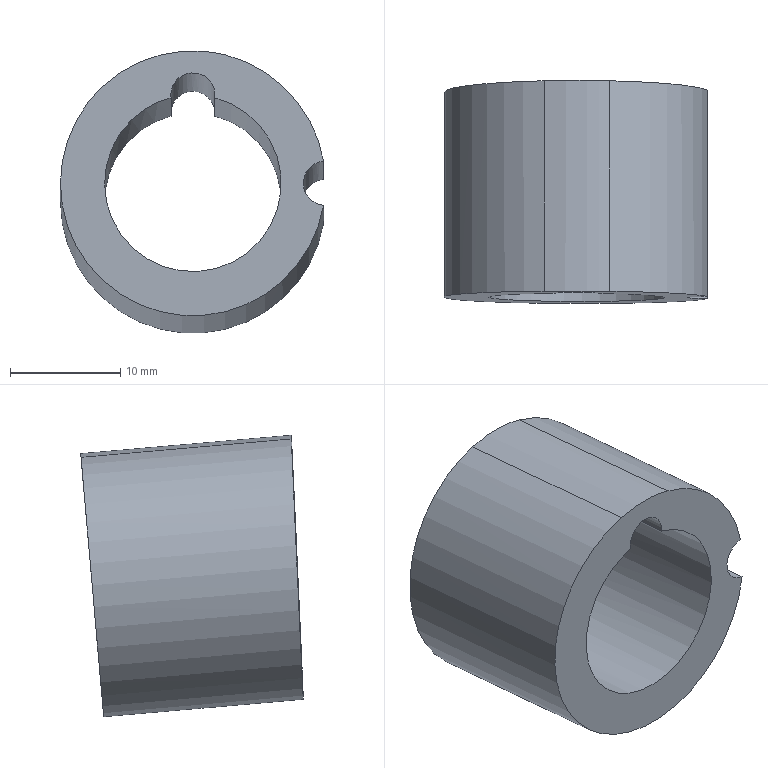Part | NX | features solid 2 | 1 solid | 8 faces | box 23.833 x 20.172 x 25.577 mm | volume 4448 mm3 | cylinder 5 | plane 2 | spline 1 | commonest cylinder face diameters 4 x2 24 x2 16 x1
STEP:
#1=CARTESIAN_POINT('',(82.605,-45.903,-31.729));
#2=VERTEX_POINT('',#1);
#3=CARTESIAN_POINT('',(91.462,-46.359,-41.358));
#4=VERTEX_POINT('',#3);
#5=CARTESIAN_POINT('',(79.629,-46.426,-43.353));
#6=DIRECTION('',(0.001957,0.999,-0.04546));
#7=DIRECTION('',(0.04675,0.04532,0.9979));
#8=AXIS2_PLACEMENT_3D('',#5,#6,#7);
#9=ELLIPSE('',#8,12.011,12.);
#10=EDGE_CURVE('',#2,#4,#9,.T.);
#11=ORIENTED_EDGE('',*,*,#10,.T.);
#12=CARTESIAN_POINT('',(91.462,-27.673,-42.993));
#13=VERTEX_POINT('',#12);
#14=CARTESIAN_POINT('',(91.462,-37.072,-42.17));
#15=DIRECTION('',(0.,0.9962,-0.08716));
#16=VECTOR('',#15,1000.);
#17=LINE('',#14,#16);
#18=EDGE_CURVE('',#4,#13,#17,.T.);
#19=ORIENTED_EDGE('',*,*,#18,.T.);
#20=CARTESIAN_POINT('',(82.605,-26.833,-33.397));
#21=VERTEX_POINT('',#20);
#22=CARTESIAN_POINT('',(79.629,-27.846,-44.978));
#23=DIRECTION('',(0.,0.9962,-0.08716));
#24=DIRECTION('',(0.,0.08716,0.9962));
#25=AXIS2_PLACEMENT_3D('',#22,#23,#24);
#26=CIRCLE('',#25,12.);
#27=EDGE_CURVE('',#21,#13,#26,.T.);
#28=ORIENTED_EDGE('',*,*,#27,.F.);
#29=CARTESIAN_POINT('',(82.605,-26.833,-33.397));
#30=DIRECTION('',(0.,-0.9962,0.08716));
#31=VECTOR('',#30,1000.);
#32=LINE('',#29,#31);
#33=EDGE_CURVE('',#21,#2,#32,.T.);
#34=ORIENTED_EDGE('',*,*,#33,.T.);
#35=EDGE_LOOP('',(#11,#19,#28,#34));
#36=FACE_BOUND('',#35,.T.);
#37=CARTESIAN_POINT('',(79.629,-27.846,-44.978));
#38=DIRECTION('',(0.,-0.9962,0.08716));
#39=DIRECTION('',(0.,-0.08716,-0.9962));
#40=AXIS2_PLACEMENT_3D('',#37,#38,#39);
#41=CYLINDRICAL_SURFACE('',#40,12.);
#42=ADVANCED_FACE('',(#36),#41,.T.);
#43=CARTESIAN_POINT('',(81.613,-46.077,-35.604));
#44=VERTEX_POINT('',#43);
#45=CARTESIAN_POINT('',(77.644,-46.07,-35.604));
#46=VERTEX_POINT('',#45);
#47=CARTESIAN_POINT('',(79.629,-46.426,-43.353));
#48=DIRECTION('',(0.001957,0.999,-0.04546));
#49=DIRECTION('',(0.04675,0.04532,0.9979));
#50=AXIS2_PLACEMENT_3D('',#47,#48,#49);
#51=ELLIPSE('',#50,8.007,8.);
#52=EDGE_CURVE('',#44,#46,#51,.T.);
#53=ORIENTED_EDGE('',*,*,#52,.F.);
#54=CARTESIAN_POINT('',(81.613,-27.171,-37.258));
#55=VERTEX_POINT('',#54);
#56=CARTESIAN_POINT('',(81.613,-27.171,-37.258));
#57=DIRECTION('',(0.,-0.9962,0.08716));
#58=VECTOR('',#57,1000.);
#59=LINE('',#56,#58);
#60=EDGE_CURVE('',#55,#44,#59,.T.);
#61=ORIENTED_EDGE('',*,*,#60,.F.);
#62=CARTESIAN_POINT('',(77.644,-27.171,-37.258));
#63=VERTEX_POINT('',#62);
#64=CARTESIAN_POINT('',(79.629,-27.846,-44.978));
#65=DIRECTION('',(0.,-0.9962,0.08716));
#66=DIRECTION('',(0.,-0.08716,-0.9962));
#67=AXIS2_PLACEMENT_3D('',#64,#65,#66);
#68=CIRCLE('',#67,8.);
#69=EDGE_CURVE('',#55,#63,#68,.F.);
#70=ORIENTED_EDGE('',*,*,#69,.T.);
#71=CARTESIAN_POINT('',(77.644,-27.171,-37.258));
#72=DIRECTION('',(0.,-0.9962,0.08716));
#73=VECTOR('',#72,1000.);
#74=LINE('',#71,#73);
#75=EDGE_CURVE('',#46,#63,#74,.F.);
#76=ORIENTED_EDGE('',*,*,#75,.F.);
#77=EDGE_LOOP('',(#53,#61,#70,#76));
#78=FACE_BOUND('',#77,.T.);
#79=CARTESIAN_POINT('',(79.629,-27.846,-44.978));
#80=DIRECTION('',(0.,-0.9962,0.08716));
#81=DIRECTION('',(0.,-0.08716,-0.9962));
#82=AXIS2_PLACEMENT_3D('',#79,#80,#81);
#83=CYLINDRICAL_SURFACE('',#82,8.);
#84=ADVANCED_FACE('',(#78),#83,.F.);
#85=CARTESIAN_POINT('',(91.462,-28.02,-46.964));
#86=VERTEX_POINT('',#85);
#87=CARTESIAN_POINT('',(91.629,-27.846,-44.978));
#88=DIRECTION('',(0.,-0.9962,0.08716));
#89=DIRECTION('',(0.,-0.08716,-0.9962));
#90=AXIS2_PLACEMENT_3D('',#87,#88,#89);
#91=CIRCLE('',#90,2.);
#92=EDGE_CURVE('',#13,#86,#91,.T.);
#93=ORIENTED_EDGE('',*,*,#92,.T.);
#94=CARTESIAN_POINT('',(76.652,-26.833,-33.397));
#95=VERTEX_POINT('',#94);
#96=CARTESIAN_POINT('',(79.629,-27.846,-44.978));
#97=DIRECTION('',(0.,0.9962,-0.08716));
#98=DIRECTION('',(0.,0.08716,0.9962));
#99=AXIS2_PLACEMENT_3D('',#96,#97,#98);
#100=CIRCLE('',#99,12.);
#101=EDGE_CURVE('',#86,#95,#100,.T.);
#102=ORIENTED_EDGE('',*,*,#101,.T.);
#103=CARTESIAN_POINT('',(76.652,-26.833,-33.397));
#104=CARTESIAN_POINT('',(78.605,-26.789,-32.899));
#105=CARTESIAN_POINT('',(80.652,-26.789,-32.899));
#106=CARTESIAN_POINT('',(82.605,-26.833,-33.397));
#107=B_SPLINE_CURVE_WITH_KNOTS('',3,(#103,#104,#105,#106),.UNSPECIFIED.,.F.,.F.,(4,4),(0.,1.),.PIECEWISE_BEZIER_KNOTS.);
#108=EDGE_CURVE('',#95,#21,#107,.T.);
#109=ORIENTED_EDGE('',*,*,#108,.T.);
#110=ORIENTED_EDGE('',*,*,#27,.T.);
#111=EDGE_LOOP('',(#93,#102,#109,#110));
#112=FACE_BOUND('',#111,.T.);
#113=CARTESIAN_POINT('',(79.629,-27.149,-37.009));
#114=DIRECTION('',(0.,-0.9962,0.08716));
#115=DIRECTION('',(0.,-0.08716,-0.9962));
#116=AXIS2_PLACEMENT_3D('',#113,#114,#115);
#117=CIRCLE('',#116,2.);
#118=EDGE_CURVE('',#55,#63,#117,.T.);
#119=ORIENTED_EDGE('',*,*,#118,.T.);
#120=ORIENTED_EDGE('',*,*,#69,.F.);
#121=EDGE_LOOP('',(#119,#120));
#122=FACE_BOUND('',#121,.T.);
#123=CARTESIAN_POINT('',(76.652,-26.833,-33.397));
#124=DIRECTION('',(0.,0.9962,-0.08716));
#125=DIRECTION('',(0.,0.08716,0.9962));
#126=AXIS2_PLACEMENT_3D('',#123,#124,#125);
#127=PLANE('',#126);
#128=ADVANCED_FACE('',(#112,#122),#127,.T.);
#129=CARTESIAN_POINT('',(91.462,-46.54,-45.343));
#130=VERTEX_POINT('',#129);
#131=CARTESIAN_POINT('',(91.629,-46.45,-43.351));
#132=DIRECTION('',(0.001957,0.999,-0.04546));
#133=DIRECTION('',(-0.04675,-0.04532,-0.9979));
#134=AXIS2_PLACEMENT_3D('',#131,#132,#133);
#135=ELLIPSE('',#134,2.002,2.);
#136=EDGE_CURVE('',#130,#4,#135,.T.);
#137=ORIENTED_EDGE('',*,*,#136,.T.);
#138=ORIENTED_EDGE('',*,*,#10,.F.);
#139=CARTESIAN_POINT('',(76.652,-45.891,-31.73));
#140=VERTEX_POINT('',#139);
#141=CARTESIAN_POINT('',(76.652,-45.891,-31.73));
#142=CARTESIAN_POINT('',(78.601,-45.872,-31.231));
#143=CARTESIAN_POINT('',(80.657,-45.876,-31.231));
#144=CARTESIAN_POINT('',(82.605,-45.903,-31.729));
#145=B_SPLINE_CURVE_WITH_KNOTS('',3,(#141,#142,#143,#144),.UNSPECIFIED.,.F.,.F.,(4,4),(0.,0.006022),.UNSPECIFIED.);
#146=EDGE_CURVE('',#140,#2,#145,.T.);
#147=ORIENTED_EDGE('',*,*,#146,.F.);
#148=CARTESIAN_POINT('',(79.629,-46.426,-43.353));
#149=DIRECTION('',(0.001957,0.999,-0.04546));
#150=DIRECTION('',(0.04675,0.04532,0.9979));
#151=AXIS2_PLACEMENT_3D('',#148,#149,#150);
#152=ELLIPSE('',#151,12.011,12.);
#153=EDGE_CURVE('',#130,#140,#152,.T.);
#154=ORIENTED_EDGE('',*,*,#153,.F.);
#155=EDGE_LOOP('',(#137,#138,#147,#154));
#156=FACE_BOUND('',#155,.T.);
#157=CARTESIAN_POINT('',(79.629,-46.062,-35.354));
#158=DIRECTION('',(0.001957,0.999,-0.04546));
#159=DIRECTION('',(-0.04675,-0.04532,-0.9979));
#160=AXIS2_PLACEMENT_3D('',#157,#158,#159);
#161=ELLIPSE('',#160,2.002,2.);
#162=EDGE_CURVE('',#46,#44,#161,.T.);
#163=ORIENTED_EDGE('',*,*,#162,.T.);
#164=ORIENTED_EDGE('',*,*,#52,.T.);
#165=EDGE_LOOP('',(#163,#164));
#166=FACE_BOUND('',#165,.T.);
#167=CARTESIAN_POINT('',(128.811,-48.589,-88.763));
#168=DIRECTION('',(0.001957,0.999,-0.04546));
#169=DIRECTION('',(0.06617,0.04523,0.9968));
#170=AXIS2_PLACEMENT_3D('',#167,#168,#169);
#171=PLANE('',#170);
#172=ADVANCED_FACE('',(#156,#166),#171,.F.);
#173=ORIENTED_EDGE('',*,*,#101,.F.);
#174=CARTESIAN_POINT('',(91.462,-37.419,-46.141));
#175=DIRECTION('',(0.,0.9962,-0.08716));
#176=VECTOR('',#175,1000.);
#177=LINE('',#174,#176);
#178=EDGE_CURVE('',#86,#130,#177,.F.);
#179=ORIENTED_EDGE('',*,*,#178,.T.);
#180=ORIENTED_EDGE('',*,*,#153,.T.);
#181=CARTESIAN_POINT('',(76.652,-26.833,-33.397));
#182=DIRECTION('',(0.,-0.9962,0.08716));
#183=VECTOR('',#182,1000.);
#184=LINE('',#181,#183);
#185=EDGE_CURVE('',#95,#140,#184,.T.);
#186=ORIENTED_EDGE('',*,*,#185,.F.);
#187=EDGE_LOOP('',(#173,#179,#180,#186));
#188=FACE_BOUND('',#187,.T.);
#189=CARTESIAN_POINT('',(79.629,-27.846,-44.978));
#190=DIRECTION('',(0.,-0.9962,0.08716));
#191=DIRECTION('',(0.,-0.08716,-0.9962));
#192=AXIS2_PLACEMENT_3D('',#189,#190,#191);
#193=CYLINDRICAL_SURFACE('',#192,12.);
#194=ADVANCED_FACE('',(#188),#193,.T.);
#195=ORIENTED_EDGE('',*,*,#146,.T.);
#196=ORIENTED_EDGE('',*,*,#33,.F.);
#197=ORIENTED_EDGE('',*,*,#108,.F.);
#198=ORIENTED_EDGE('',*,*,#185,.T.);
#199=EDGE_LOOP('',(#195,#196,#197,#198));
#200=FACE_BOUND('',#199,.T.);
#201=CARTESIAN_POINT('',(76.652,-26.833,-33.397));
#202=CARTESIAN_POINT('',(76.652,-46.029,-31.718));
#203=CARTESIAN_POINT('',(78.605,-26.789,-32.899));
#204=CARTESIAN_POINT('',(78.605,-45.985,-31.22));
#205=CARTESIAN_POINT('',(80.652,-26.789,-32.899));
#206=CARTESIAN_POINT('',(80.652,-45.985,-31.22));
#207=CARTESIAN_POINT('',(82.605,-26.833,-33.397));
#208=CARTESIAN_POINT('',(82.605,-46.029,-31.718));
#209=B_SPLINE_SURFACE_WITH_KNOTS('',3,1,((#201,#202),(#203,#204),(#205,#206),(#207,#208)),.SURF_OF_LINEAR_EXTRUSION.,.F.,.F.,.F.,(4,4),(2,2),(0.,1.),(0.,1.),.PIECEWISE_BEZIER_KNOTS.);
#210=ADVANCED_FACE('',(#200),#209,.F.);
#211=ORIENTED_EDGE('',*,*,#75,.T.);
#212=ORIENTED_EDGE('',*,*,#118,.F.);
#213=ORIENTED_EDGE('',*,*,#60,.T.);
#214=ORIENTED_EDGE('',*,*,#162,.F.);
#215=EDGE_LOOP('',(#211,#212,#213,#214));
#216=FACE_BOUND('',#215,.T.);
#217=CARTESIAN_POINT('',(79.629,-47.073,-35.266));
#218=DIRECTION('',(0.,0.9962,-0.08716));
#219=DIRECTION('',(0.,0.08716,0.9962));
#220=AXIS2_PLACEMENT_3D('',#217,#218,#219);
#221=CYLINDRICAL_SURFACE('',#220,2.);
#222=ADVANCED_FACE('',(#216),#221,.F.);
#223=ORIENTED_EDGE('',*,*,#136,.F.);
#224=ORIENTED_EDGE('',*,*,#178,.F.);
#225=ORIENTED_EDGE('',*,*,#92,.F.);
#226=ORIENTED_EDGE('',*,*,#18,.F.);
#227=EDGE_LOOP('',(#223,#224,#225,#226));
#228=FACE_BOUND('',#227,.T.);
#229=CARTESIAN_POINT('',(91.629,-47.77,-43.235));
#230=DIRECTION('',(0.,0.9962,-0.08716));
#231=DIRECTION('',(0.,0.08716,0.9962));
#232=AXIS2_PLACEMENT_3D('',#229,#230,#231);
#233=CYLINDRICAL_SURFACE('',#232,2.);
#234=ADVANCED_FACE('',(#228),#233,.F.);
#235=CLOSED_SHELL('',(#42,#84,#128,#172,#194,#210,#222,#234));
#236=MANIFOLD_SOLID_BREP('',#235);
#237=(LENGTH_UNIT()NAMED_UNIT(*)SI_UNIT(.MILLI.,.METRE.));
#238=UNCERTAINTY_MEASURE_WITH_UNIT(LENGTH_MEASURE(0.0508),#237,'','');
#239=(NAMED_UNIT(*)PLANE_ANGLE_UNIT()SI_UNIT($,.RADIAN.));
#240=(NAMED_UNIT(*)SI_UNIT($,.STERADIAN.)SOLID_ANGLE_UNIT());
#241=(GEOMETRIC_REPRESENTATION_CONTEXT(3)GLOBAL_UNCERTAINTY_ASSIGNED_CONTEXT((#238))GLOBAL_UNIT_ASSIGNED_CONTEXT((#237,#239,#240))REPRESENTATION_CONTEXT('',''));
#242=ADVANCED_BREP_SHAPE_REPRESENTATION('',(#236),#241);